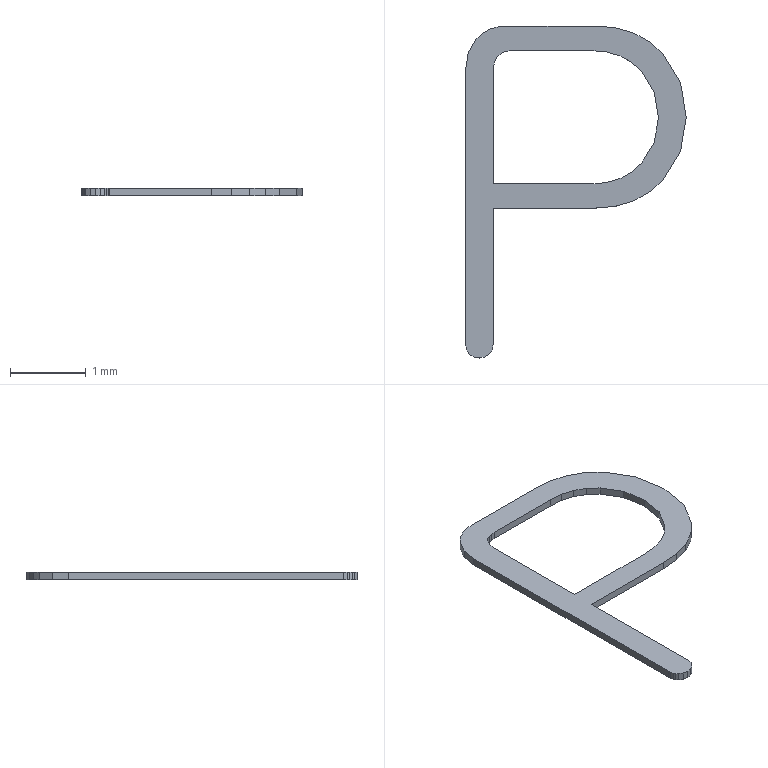Part | STEP file | PART235.stp | 1 solid | 57 faces | box 2.914 x 4.388 x 0.1 mm | volume 0.3534 mm3 | plane 57